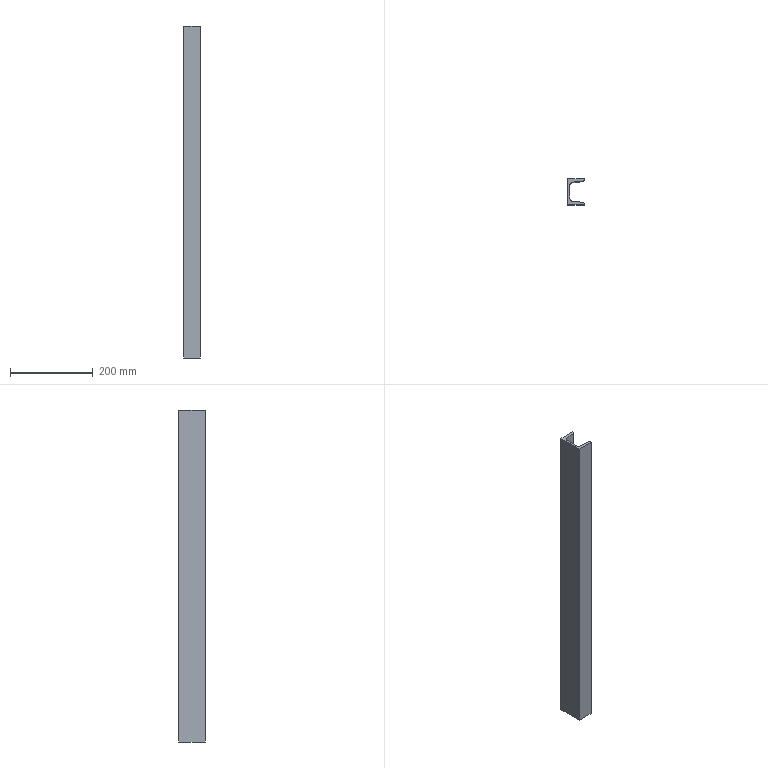Part | STEP file | 750038449 | 1 solid | 14 faces | box 40 x 63 x 800 mm | volume 675654 mm3 | plane 10 | cylinder 4 | commonest cylinder face diameters 7.6 x2 15 x2
STEP:
#1=CARTESIAN_POINT('',(0.,0.,800.));
#2=VERTEX_POINT('',#1);
#3=CARTESIAN_POINT('',(0.,0.,0.));
#4=VERTEX_POINT('',#3);
#5=CARTESIAN_POINT('',(0.,0.,800.));
#6=DIRECTION('',(0.,0.,-1.));
#7=VECTOR('',#6,1000.);
#8=LINE('',#5,#7);
#9=EDGE_CURVE('',#2,#4,#8,.T.);
#10=ORIENTED_EDGE('',*,*,#9,.F.);
#11=CARTESIAN_POINT('',(0.,63.,800.));
#12=VERTEX_POINT('',#11);
#13=CARTESIAN_POINT('',(0.,63.,800.));
#14=DIRECTION('',(0.,-1.,0.));
#15=VECTOR('',#14,1000.);
#16=LINE('',#13,#15);
#17=EDGE_CURVE('',#12,#2,#16,.T.);
#18=ORIENTED_EDGE('',*,*,#17,.F.);
#19=CARTESIAN_POINT('',(0.,63.,0.));
#20=VERTEX_POINT('',#19);
#21=CARTESIAN_POINT('',(0.,63.,800.));
#22=DIRECTION('',(0.,0.,1.));
#23=VECTOR('',#22,1000.);
#24=LINE('',#21,#23);
#25=EDGE_CURVE('',#20,#12,#24,.T.);
#26=ORIENTED_EDGE('',*,*,#25,.F.);
#27=CARTESIAN_POINT('',(0.,63.,0.));
#28=DIRECTION('',(0.,1.,0.));
#29=VECTOR('',#28,1000.);
#30=LINE('',#27,#29);
#31=EDGE_CURVE('',#4,#20,#30,.T.);
#32=ORIENTED_EDGE('',*,*,#31,.F.);
#33=EDGE_LOOP('',(#10,#18,#26,#32));
#34=FACE_OUTER_BOUND('',#33,.T.);
#35=CARTESIAN_POINT('',(0.,63.,800.));
#36=DIRECTION('',(1.,0.,0.));
#37=DIRECTION('',(0.,0.,-1.));
#38=AXIS2_PLACEMENT_3D('',#35,#36,#37);
#39=PLANE('',#38);
#40=ADVANCED_FACE('',(#34),#39,.F.);
#41=CARTESIAN_POINT('',(40.,63.,0.));
#42=VERTEX_POINT('',#41);
#43=CARTESIAN_POINT('',(36.2,63.,0.));
#44=DIRECTION('',(-1.,0.,0.));
#45=VECTOR('',#44,1000.);
#46=LINE('',#43,#45);
#47=EDGE_CURVE('',#42,#20,#46,.T.);
#48=ORIENTED_EDGE('',*,*,#47,.F.);
#49=CARTESIAN_POINT('',(40.,60.699,0.));
#50=VERTEX_POINT('',#49);
#51=CARTESIAN_POINT('',(40.,2.301,0.));
#52=DIRECTION('',(0.,1.,0.));
#53=VECTOR('',#52,1000.);
#54=LINE('',#51,#53);
#55=EDGE_CURVE('',#50,#42,#54,.T.);
#56=ORIENTED_EDGE('',*,*,#55,.F.);
#57=CARTESIAN_POINT('',(36.578,56.918,0.));
#58=VERTEX_POINT('',#57);
#59=CARTESIAN_POINT('',(36.2,60.699,0.));
#60=DIRECTION('',(0.,0.,1.));
#61=DIRECTION('',(-1.,0.,0.));
#62=AXIS2_PLACEMENT_3D('',#59,#60,#61);
#63=CIRCLE('',#62,3.8);
#64=EDGE_CURVE('',#58,#50,#63,.T.);
#65=ORIENTED_EDGE('',*,*,#64,.F.);
#66=CARTESIAN_POINT('',(11.554,54.415,0.));
#67=VERTEX_POINT('',#66);
#68=CARTESIAN_POINT('',(11.554,54.415,0.));
#69=DIRECTION('',(0.995,0.0995,0.));
#70=VECTOR('',#69,1000.);
#71=LINE('',#68,#70);
#72=EDGE_CURVE('',#67,#58,#71,.T.);
#73=ORIENTED_EDGE('',*,*,#72,.F.);
#74=CARTESIAN_POINT('',(4.8,46.953,0.));
#75=VERTEX_POINT('',#74);
#76=CARTESIAN_POINT('',(12.3,46.953,0.));
#77=DIRECTION('',(0.,0.,-1.));
#78=DIRECTION('',(-1.,0.,0.));
#79=AXIS2_PLACEMENT_3D('',#76,#77,#78);
#80=CIRCLE('',#79,7.5);
#81=EDGE_CURVE('',#75,#67,#80,.T.);
#82=ORIENTED_EDGE('',*,*,#81,.F.);
#83=CARTESIAN_POINT('',(4.8,16.047,0.));
#84=VERTEX_POINT('',#83);
#85=CARTESIAN_POINT('',(4.8,2.301,0.));
#86=DIRECTION('',(0.,1.,0.));
#87=VECTOR('',#86,1000.);
#88=LINE('',#85,#87);
#89=EDGE_CURVE('',#84,#75,#88,.T.);
#90=ORIENTED_EDGE('',*,*,#89,.F.);
#91=CARTESIAN_POINT('',(11.554,8.585,0.));
#92=VERTEX_POINT('',#91);
#93=CARTESIAN_POINT('',(12.3,16.047,0.));
#94=DIRECTION('',(0.,0.,-1.));
#95=DIRECTION('',(-1.,0.,0.));
#96=AXIS2_PLACEMENT_3D('',#93,#94,#95);
#97=CIRCLE('',#96,7.5);
#98=EDGE_CURVE('',#92,#84,#97,.T.);
#99=ORIENTED_EDGE('',*,*,#98,.F.);
#100=CARTESIAN_POINT('',(36.578,6.082,0.));
#101=VERTEX_POINT('',#100);
#102=CARTESIAN_POINT('',(36.578,6.082,0.));
#103=DIRECTION('',(-0.995,0.0995,0.));
#104=VECTOR('',#103,1000.);
#105=LINE('',#102,#104);
#106=EDGE_CURVE('',#101,#92,#105,.T.);
#107=ORIENTED_EDGE('',*,*,#106,.F.);
#108=CARTESIAN_POINT('',(40.,2.301,0.));
#109=VERTEX_POINT('',#108);
#110=CARTESIAN_POINT('',(36.2,2.301,0.));
#111=DIRECTION('',(0.,0.,1.));
#112=DIRECTION('',(-1.,0.,0.));
#113=AXIS2_PLACEMENT_3D('',#110,#111,#112);
#114=CIRCLE('',#113,3.8);
#115=EDGE_CURVE('',#109,#101,#114,.T.);
#116=ORIENTED_EDGE('',*,*,#115,.F.);
#117=CARTESIAN_POINT('',(40.,0.,0.));
#118=VERTEX_POINT('',#117);
#119=CARTESIAN_POINT('',(40.,2.301,0.));
#120=DIRECTION('',(0.,1.,0.));
#121=VECTOR('',#120,1000.);
#122=LINE('',#119,#121);
#123=EDGE_CURVE('',#118,#109,#122,.T.);
#124=ORIENTED_EDGE('',*,*,#123,.F.);
#125=CARTESIAN_POINT('',(36.2,0.,0.));
#126=DIRECTION('',(1.,0.,0.));
#127=VECTOR('',#126,1000.);
#128=LINE('',#125,#127);
#129=EDGE_CURVE('',#4,#118,#128,.T.);
#130=ORIENTED_EDGE('',*,*,#129,.F.);
#131=ORIENTED_EDGE('',*,*,#31,.T.);
#132=EDGE_LOOP('',(#48,#56,#65,#73,#82,#90,#99,#107,#116,#124,#130,#131));
#133=FACE_OUTER_BOUND('',#132,.T.);
#134=CARTESIAN_POINT('',(36.2,2.301,0.));
#135=DIRECTION('',(0.,0.,1.));
#136=DIRECTION('',(1.,0.,0.));
#137=AXIS2_PLACEMENT_3D('',#134,#135,#136);
#138=PLANE('',#137);
#139=ADVANCED_FACE('',(#133),#138,.F.);
#140=CARTESIAN_POINT('',(40.,0.,800.));
#141=VERTEX_POINT('',#140);
#142=CARTESIAN_POINT('',(40.,0.,800.));
#143=DIRECTION('',(0.,0.,-1.));
#144=VECTOR('',#143,1000.);
#145=LINE('',#142,#144);
#146=EDGE_CURVE('',#141,#118,#145,.T.);
#147=ORIENTED_EDGE('',*,*,#146,.F.);
#148=CARTESIAN_POINT('',(0.,0.,800.));
#149=DIRECTION('',(1.,0.,0.));
#150=VECTOR('',#149,1000.);
#151=LINE('',#148,#150);
#152=EDGE_CURVE('',#2,#141,#151,.T.);
#153=ORIENTED_EDGE('',*,*,#152,.F.);
#154=ORIENTED_EDGE('',*,*,#9,.T.);
#155=ORIENTED_EDGE('',*,*,#129,.T.);
#156=EDGE_LOOP('',(#147,#153,#154,#155));
#157=FACE_OUTER_BOUND('',#156,.T.);
#158=CARTESIAN_POINT('',(0.,0.,800.));
#159=DIRECTION('',(0.,1.,0.));
#160=DIRECTION('',(0.,0.,1.));
#161=AXIS2_PLACEMENT_3D('',#158,#159,#160);
#162=PLANE('',#161);
#163=ADVANCED_FACE('',(#157),#162,.F.);
#164=CARTESIAN_POINT('',(40.,60.699,800.));
#165=VERTEX_POINT('',#164);
#166=CARTESIAN_POINT('',(40.,63.,800.));
#167=VERTEX_POINT('',#166);
#168=CARTESIAN_POINT('',(40.,2.301,800.));
#169=DIRECTION('',(0.,1.,0.));
#170=VECTOR('',#169,1000.);
#171=LINE('',#168,#170);
#172=EDGE_CURVE('',#165,#167,#171,.T.);
#173=ORIENTED_EDGE('',*,*,#172,.T.);
#174=CARTESIAN_POINT('',(36.2,63.,800.));
#175=DIRECTION('',(-1.,0.,0.));
#176=VECTOR('',#175,1000.);
#177=LINE('',#174,#176);
#178=EDGE_CURVE('',#167,#12,#177,.T.);
#179=ORIENTED_EDGE('',*,*,#178,.T.);
#180=ORIENTED_EDGE('',*,*,#17,.T.);
#181=ORIENTED_EDGE('',*,*,#152,.T.);
#182=CARTESIAN_POINT('',(40.,2.301,800.));
#183=VERTEX_POINT('',#182);
#184=CARTESIAN_POINT('',(40.,2.301,800.));
#185=DIRECTION('',(0.,1.,0.));
#186=VECTOR('',#185,1000.);
#187=LINE('',#184,#186);
#188=EDGE_CURVE('',#141,#183,#187,.T.);
#189=ORIENTED_EDGE('',*,*,#188,.T.);
#190=CARTESIAN_POINT('',(36.578,6.082,800.));
#191=VERTEX_POINT('',#190);
#192=CARTESIAN_POINT('',(36.2,2.301,800.));
#193=DIRECTION('',(0.,0.,1.));
#194=DIRECTION('',(-1.,0.,0.));
#195=AXIS2_PLACEMENT_3D('',#192,#193,#194);
#196=CIRCLE('',#195,3.8);
#197=EDGE_CURVE('',#183,#191,#196,.T.);
#198=ORIENTED_EDGE('',*,*,#197,.T.);
#199=CARTESIAN_POINT('',(11.554,8.585,800.));
#200=VERTEX_POINT('',#199);
#201=CARTESIAN_POINT('',(36.578,6.082,800.));
#202=DIRECTION('',(-0.995,0.0995,0.));
#203=VECTOR('',#202,1000.);
#204=LINE('',#201,#203);
#205=EDGE_CURVE('',#191,#200,#204,.T.);
#206=ORIENTED_EDGE('',*,*,#205,.T.);
#207=CARTESIAN_POINT('',(4.8,16.047,800.));
#208=VERTEX_POINT('',#207);
#209=CARTESIAN_POINT('',(12.3,16.047,800.));
#210=DIRECTION('',(0.,0.,-1.));
#211=DIRECTION('',(-1.,0.,0.));
#212=AXIS2_PLACEMENT_3D('',#209,#210,#211);
#213=CIRCLE('',#212,7.5);
#214=EDGE_CURVE('',#200,#208,#213,.T.);
#215=ORIENTED_EDGE('',*,*,#214,.T.);
#216=CARTESIAN_POINT('',(4.8,46.953,800.));
#217=VERTEX_POINT('',#216);
#218=CARTESIAN_POINT('',(4.8,2.301,800.));
#219=DIRECTION('',(0.,1.,0.));
#220=VECTOR('',#219,1000.);
#221=LINE('',#218,#220);
#222=EDGE_CURVE('',#208,#217,#221,.T.);
#223=ORIENTED_EDGE('',*,*,#222,.T.);
#224=CARTESIAN_POINT('',(11.554,54.415,800.));
#225=VERTEX_POINT('',#224);
#226=CARTESIAN_POINT('',(12.3,46.953,800.));
#227=DIRECTION('',(0.,0.,-1.));
#228=DIRECTION('',(-1.,0.,0.));
#229=AXIS2_PLACEMENT_3D('',#226,#227,#228);
#230=CIRCLE('',#229,7.5);
#231=EDGE_CURVE('',#217,#225,#230,.T.);
#232=ORIENTED_EDGE('',*,*,#231,.T.);
#233=CARTESIAN_POINT('',(36.578,56.918,800.));
#234=VERTEX_POINT('',#233);
#235=CARTESIAN_POINT('',(11.554,54.415,800.));
#236=DIRECTION('',(0.995,0.0995,0.));
#237=VECTOR('',#236,1000.);
#238=LINE('',#235,#237);
#239=EDGE_CURVE('',#225,#234,#238,.T.);
#240=ORIENTED_EDGE('',*,*,#239,.T.);
#241=CARTESIAN_POINT('',(36.2,60.699,800.));
#242=DIRECTION('',(0.,0.,1.));
#243=DIRECTION('',(-1.,0.,0.));
#244=AXIS2_PLACEMENT_3D('',#241,#242,#243);
#245=CIRCLE('',#244,3.8);
#246=EDGE_CURVE('',#234,#165,#245,.T.);
#247=ORIENTED_EDGE('',*,*,#246,.T.);
#248=EDGE_LOOP('',(#173,#179,#180,#181,#189,#198,#206,#215,#223,#232,#240,#247));
#249=FACE_OUTER_BOUND('',#248,.T.);
#250=CARTESIAN_POINT('',(36.2,2.301,800.));
#251=DIRECTION('',(0.,0.,1.));
#252=DIRECTION('',(1.,0.,0.));
#253=AXIS2_PLACEMENT_3D('',#250,#251,#252);
#254=PLANE('',#253);
#255=ADVANCED_FACE('',(#249),#254,.T.);
#256=ORIENTED_EDGE('',*,*,#25,.T.);
#257=ORIENTED_EDGE('',*,*,#178,.F.);
#258=CARTESIAN_POINT('',(40.,63.,800.));
#259=DIRECTION('',(0.,0.,1.));
#260=VECTOR('',#259,1000.);
#261=LINE('',#258,#260);
#262=EDGE_CURVE('',#42,#167,#261,.T.);
#263=ORIENTED_EDGE('',*,*,#262,.F.);
#264=ORIENTED_EDGE('',*,*,#47,.T.);
#265=EDGE_LOOP('',(#256,#257,#263,#264));
#266=FACE_OUTER_BOUND('',#265,.T.);
#267=CARTESIAN_POINT('',(40.,63.,800.));
#268=DIRECTION('',(0.,-1.,0.));
#269=DIRECTION('',(0.,0.,-1.));
#270=AXIS2_PLACEMENT_3D('',#267,#268,#269);
#271=PLANE('',#270);
#272=ADVANCED_FACE('',(#266),#271,.F.);
#273=ORIENTED_EDGE('',*,*,#262,.T.);
#274=ORIENTED_EDGE('',*,*,#172,.F.);
#275=CARTESIAN_POINT('',(40.,60.699,800.));
#276=DIRECTION('',(0.,0.,1.));
#277=VECTOR('',#276,1000.);
#278=LINE('',#275,#277);
#279=EDGE_CURVE('',#50,#165,#278,.T.);
#280=ORIENTED_EDGE('',*,*,#279,.F.);
#281=ORIENTED_EDGE('',*,*,#55,.T.);
#282=EDGE_LOOP('',(#273,#274,#280,#281));
#283=FACE_OUTER_BOUND('',#282,.T.);
#284=CARTESIAN_POINT('',(40.,60.699,800.));
#285=DIRECTION('',(-1.,0.,0.));
#286=DIRECTION('',(0.,-1.,0.));
#287=AXIS2_PLACEMENT_3D('',#284,#285,#286);
#288=PLANE('',#287);
#289=ADVANCED_FACE('',(#283),#288,.F.);
#290=ORIENTED_EDGE('',*,*,#246,.F.);
#291=CARTESIAN_POINT('',(36.578,56.918,800.));
#292=DIRECTION('',(0.,0.,-1.));
#293=VECTOR('',#292,1000.);
#294=LINE('',#291,#293);
#295=EDGE_CURVE('',#234,#58,#294,.T.);
#296=ORIENTED_EDGE('',*,*,#295,.T.);
#297=ORIENTED_EDGE('',*,*,#64,.T.);
#298=ORIENTED_EDGE('',*,*,#279,.T.);
#299=EDGE_LOOP('',(#290,#296,#297,#298));
#300=FACE_OUTER_BOUND('',#299,.T.);
#301=CARTESIAN_POINT('',(36.2,60.699,800.));
#302=DIRECTION('',(0.,0.,-1.));
#303=DIRECTION('',(-1.,0.,0.));
#304=AXIS2_PLACEMENT_3D('',#301,#302,#303);
#305=CYLINDRICAL_SURFACE('',#304,3.8);
#306=ADVANCED_FACE('',(#300),#305,.T.);
#307=ORIENTED_EDGE('',*,*,#295,.F.);
#308=ORIENTED_EDGE('',*,*,#239,.F.);
#309=CARTESIAN_POINT('',(11.554,54.415,800.));
#310=DIRECTION('',(0.,0.,1.));
#311=VECTOR('',#310,1000.);
#312=LINE('',#309,#311);
#313=EDGE_CURVE('',#67,#225,#312,.T.);
#314=ORIENTED_EDGE('',*,*,#313,.F.);
#315=ORIENTED_EDGE('',*,*,#72,.T.);
#316=EDGE_LOOP('',(#307,#308,#314,#315));
#317=FACE_OUTER_BOUND('',#316,.T.);
#318=CARTESIAN_POINT('',(11.554,54.415,800.));
#319=DIRECTION('',(-0.0995,0.995,0.));
#320=DIRECTION('',(-0.995,-0.0995,0.));
#321=AXIS2_PLACEMENT_3D('',#318,#319,#320);
#322=PLANE('',#321);
#323=ADVANCED_FACE('',(#317),#322,.F.);
#324=ORIENTED_EDGE('',*,*,#313,.T.);
#325=ORIENTED_EDGE('',*,*,#231,.F.);
#326=CARTESIAN_POINT('',(4.8,46.953,800.));
#327=DIRECTION('',(0.,0.,1.));
#328=VECTOR('',#327,1000.);
#329=LINE('',#326,#328);
#330=EDGE_CURVE('',#75,#217,#329,.T.);
#331=ORIENTED_EDGE('',*,*,#330,.F.);
#332=ORIENTED_EDGE('',*,*,#81,.T.);
#333=EDGE_LOOP('',(#324,#325,#331,#332));
#334=FACE_OUTER_BOUND('',#333,.T.);
#335=CARTESIAN_POINT('',(12.3,46.953,800.));
#336=DIRECTION('',(0.,0.,-1.));
#337=DIRECTION('',(-1.,0.,0.));
#338=AXIS2_PLACEMENT_3D('',#335,#336,#337);
#339=CYLINDRICAL_SURFACE('',#338,7.5);
#340=ADVANCED_FACE('',(#334),#339,.F.);
#341=ORIENTED_EDGE('',*,*,#330,.T.);
#342=ORIENTED_EDGE('',*,*,#222,.F.);
#343=CARTESIAN_POINT('',(4.8,16.047,800.));
#344=DIRECTION('',(0.,0.,1.));
#345=VECTOR('',#344,1000.);
#346=LINE('',#343,#345);
#347=EDGE_CURVE('',#84,#208,#346,.T.);
#348=ORIENTED_EDGE('',*,*,#347,.F.);
#349=ORIENTED_EDGE('',*,*,#89,.T.);
#350=EDGE_LOOP('',(#341,#342,#348,#349));
#351=FACE_OUTER_BOUND('',#350,.T.);
#352=CARTESIAN_POINT('',(4.8,16.047,800.));
#353=DIRECTION('',(-1.,0.,0.));
#354=DIRECTION('',(0.,-1.,0.));
#355=AXIS2_PLACEMENT_3D('',#352,#353,#354);
#356=PLANE('',#355);
#357=ADVANCED_FACE('',(#351),#356,.F.);
#358=ORIENTED_EDGE('',*,*,#347,.T.);
#359=ORIENTED_EDGE('',*,*,#214,.F.);
#360=CARTESIAN_POINT('',(11.554,8.585,800.));
#361=DIRECTION('',(0.,0.,1.));
#362=VECTOR('',#361,1000.);
#363=LINE('',#360,#362);
#364=EDGE_CURVE('',#92,#200,#363,.T.);
#365=ORIENTED_EDGE('',*,*,#364,.F.);
#366=ORIENTED_EDGE('',*,*,#98,.T.);
#367=EDGE_LOOP('',(#358,#359,#365,#366));
#368=FACE_OUTER_BOUND('',#367,.T.);
#369=CARTESIAN_POINT('',(12.3,16.047,800.));
#370=DIRECTION('',(0.,0.,-1.));
#371=DIRECTION('',(-1.,0.,0.));
#372=AXIS2_PLACEMENT_3D('',#369,#370,#371);
#373=CYLINDRICAL_SURFACE('',#372,7.5);
#374=ADVANCED_FACE('',(#368),#373,.F.);
#375=ORIENTED_EDGE('',*,*,#364,.T.);
#376=ORIENTED_EDGE('',*,*,#205,.F.);
#377=CARTESIAN_POINT('',(36.578,6.082,800.));
#378=DIRECTION('',(0.,0.,1.));
#379=VECTOR('',#378,1000.);
#380=LINE('',#377,#379);
#381=EDGE_CURVE('',#101,#191,#380,.T.);
#382=ORIENTED_EDGE('',*,*,#381,.F.);
#383=ORIENTED_EDGE('',*,*,#106,.T.);
#384=EDGE_LOOP('',(#375,#376,#382,#383));
#385=FACE_OUTER_BOUND('',#384,.T.);
#386=CARTESIAN_POINT('',(36.578,6.082,800.));
#387=DIRECTION('',(-0.0995,-0.995,0.));
#388=DIRECTION('',(0.995,-0.0995,0.));
#389=AXIS2_PLACEMENT_3D('',#386,#387,#388);
#390=PLANE('',#389);
#391=ADVANCED_FACE('',(#385),#390,.F.);
#392=ORIENTED_EDGE('',*,*,#197,.F.);
#393=CARTESIAN_POINT('',(40.,2.301,800.));
#394=DIRECTION('',(0.,0.,-1.));
#395=VECTOR('',#394,1000.);
#396=LINE('',#393,#395);
#397=EDGE_CURVE('',#183,#109,#396,.T.);
#398=ORIENTED_EDGE('',*,*,#397,.T.);
#399=ORIENTED_EDGE('',*,*,#115,.T.);
#400=ORIENTED_EDGE('',*,*,#381,.T.);
#401=EDGE_LOOP('',(#392,#398,#399,#400));
#402=FACE_OUTER_BOUND('',#401,.T.);
#403=CARTESIAN_POINT('',(36.2,2.301,800.));
#404=DIRECTION('',(0.,0.,-1.));
#405=DIRECTION('',(-1.,0.,0.));
#406=AXIS2_PLACEMENT_3D('',#403,#404,#405);
#407=CYLINDRICAL_SURFACE('',#406,3.8);
#408=ADVANCED_FACE('',(#402),#407,.T.);
#409=ORIENTED_EDGE('',*,*,#397,.F.);
#410=ORIENTED_EDGE('',*,*,#188,.F.);
#411=ORIENTED_EDGE('',*,*,#146,.T.);
#412=ORIENTED_EDGE('',*,*,#123,.T.);
#413=EDGE_LOOP('',(#409,#410,#411,#412));
#414=FACE_OUTER_BOUND('',#413,.T.);
#415=CARTESIAN_POINT('',(40.,0.,800.));
#416=DIRECTION('',(-1.,0.,0.));
#417=DIRECTION('',(0.,0.,1.));
#418=AXIS2_PLACEMENT_3D('',#415,#416,#417);
#419=PLANE('',#418);
#420=ADVANCED_FACE('',(#414),#419,.F.);
#421=CLOSED_SHELL('',(#40,#139,#163,#255,#272,#289,#306,#323,#340,#357,#374,#391,#408,#420));
#422=MANIFOLD_SOLID_BREP('',#421);
#423=CARTESIAN_POINT('',(0.,0.,0.));
#424=DIRECTION('',(0.,0.,1.));
#425=DIRECTION('',(1.,0.,0.));
#426=AXIS2_PLACEMENT_3D('',#423,#424,#425);
#427=(LENGTH_UNIT()NAMED_UNIT(*)SI_UNIT(.MILLI.,.METRE.));
#428=UNCERTAINTY_MEASURE_WITH_UNIT(LENGTH_MEASURE(0.00001),#427,'','');
#429=(NAMED_UNIT(*)PLANE_ANGLE_UNIT()SI_UNIT($,.RADIAN.));
#430=(NAMED_UNIT(*)SI_UNIT($,.STERADIAN.)SOLID_ANGLE_UNIT());
#431=(GEOMETRIC_REPRESENTATION_CONTEXT(3)GLOBAL_UNCERTAINTY_ASSIGNED_CONTEXT((#428))GLOBAL_UNIT_ASSIGNED_CONTEXT((#427,#429,#430))REPRESENTATION_CONTEXT('',''));
#432=ADVANCED_BREP_SHAPE_REPRESENTATION('',(#422,#426),#431);